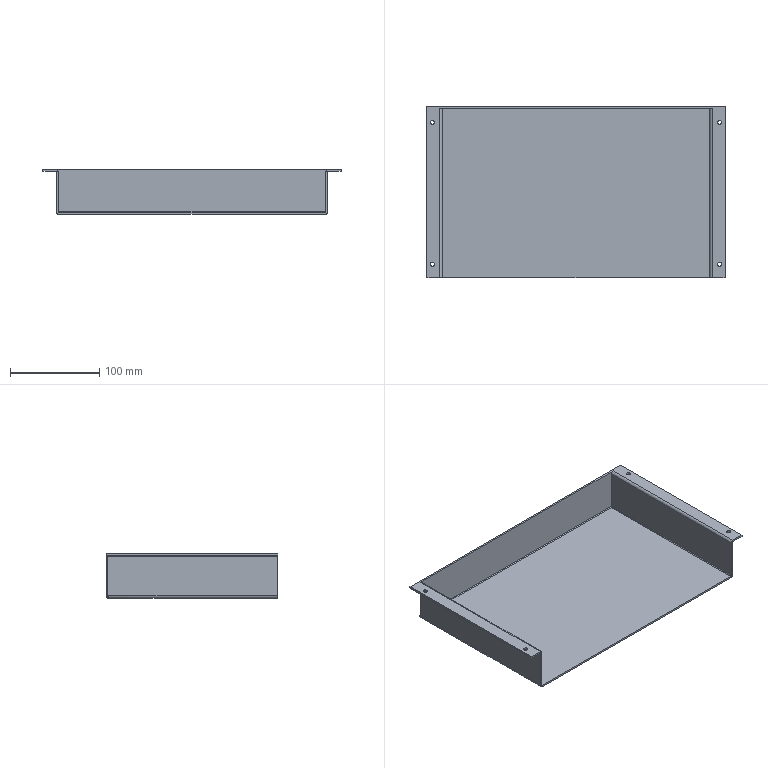Part | STEP file | Manual box | 1 solid | 48 faces | box 334 x 192 x 50 mm | volume 192178 mm3 | cylinder 22 | plane 14 | spline 12 | commonest cylinder face diameters 4.5 x8 1.473 x5 5.473 x5 2 x4